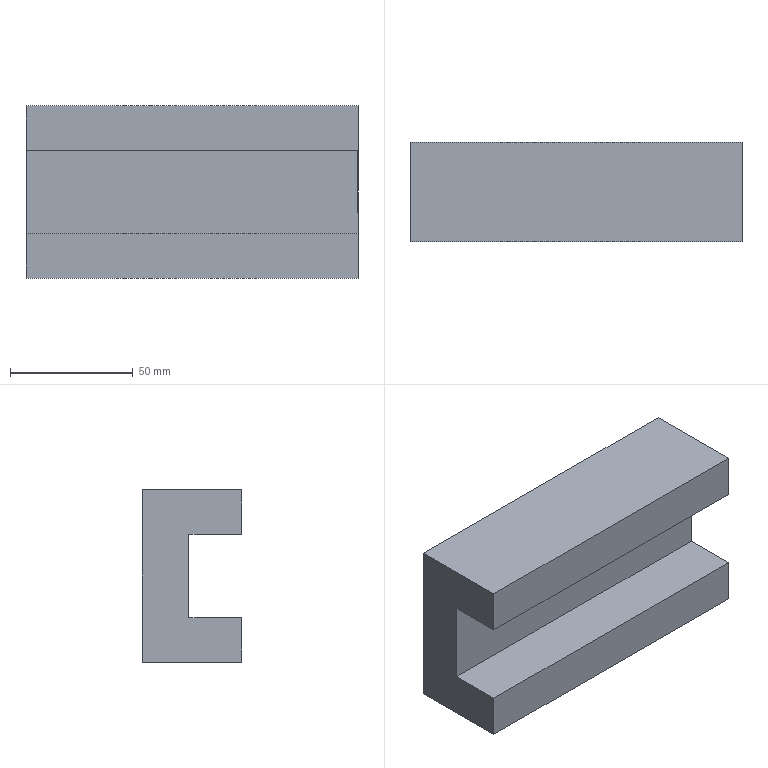Part | SolidWorks | features Cut 2, Extrusion 1 | 1 solid | 22 faces | box 135 x 40.5 x 70 mm | volume 280823 mm3 | plane 14 | cylinder 8 | commonest cylinder face diameters 8 x8
STEP:
#1=CARTESIAN_POINT('',(31.5,24.5,-14.));
#2=VERTEX_POINT('',#1);
#3=CARTESIAN_POINT('',(31.5,24.5,-6.));
#4=VERTEX_POINT('',#3);
#5=CARTESIAN_POINT('',(31.5,24.5,-10.));
#6=DIRECTION('',(0.,1.,0.));
#7=DIRECTION('',(0.,0.,1.));
#8=AXIS2_PLACEMENT_3D('',#5,#6,#7);
#9=CIRCLE('',#8,4.);
#10=EDGE_CURVE('',#2,#4,#9,.T.);
#11=ORIENTED_EDGE('',*,*,#10,.F.);
#12=CARTESIAN_POINT('',(31.5,40.5,-14.));
#13=VERTEX_POINT('',#12);
#14=CARTESIAN_POINT('',(31.5,24.5,-14.));
#15=DIRECTION('',(0.,1.,0.));
#16=VECTOR('',#15,1000.);
#17=LINE('',#14,#16);
#18=EDGE_CURVE('',#2,#13,#17,.T.);
#19=ORIENTED_EDGE('',*,*,#18,.T.);
#20=CARTESIAN_POINT('',(31.5,40.5,-6.));
#21=VERTEX_POINT('',#20);
#22=CARTESIAN_POINT('',(31.5,40.5,-10.));
#23=DIRECTION('',(0.,1.,0.));
#24=DIRECTION('',(0.,0.,1.));
#25=AXIS2_PLACEMENT_3D('',#22,#23,#24);
#26=CIRCLE('',#25,4.);
#27=EDGE_CURVE('',#13,#21,#26,.T.);
#28=ORIENTED_EDGE('',*,*,#27,.T.);
#29=CARTESIAN_POINT('',(31.5,24.5,-6.));
#30=DIRECTION('',(0.,1.,0.));
#31=VECTOR('',#30,1000.);
#32=LINE('',#29,#31);
#33=EDGE_CURVE('',#4,#21,#32,.T.);
#34=ORIENTED_EDGE('',*,*,#33,.F.);
#35=EDGE_LOOP('',(#11,#19,#28,#34));
#36=FACE_OUTER_BOUND('',#35,.T.);
#37=CARTESIAN_POINT('',(31.5,24.5,-10.));
#38=DIRECTION('',(0.,1.,0.));
#39=DIRECTION('',(0.,0.,1.));
#40=AXIS2_PLACEMENT_3D('',#37,#38,#39);
#41=CYLINDRICAL_SURFACE('',#40,4.);
#42=ADVANCED_FACE('',(#36),#41,.F.);
#43=CARTESIAN_POINT('',(31.5,24.5,-64.));
#44=VERTEX_POINT('',#43);
#45=CARTESIAN_POINT('',(31.5,24.5,-56.));
#46=VERTEX_POINT('',#45);
#47=CARTESIAN_POINT('',(31.5,24.5,-60.));
#48=DIRECTION('',(0.,1.,0.));
#49=DIRECTION('',(0.,0.,1.));
#50=AXIS2_PLACEMENT_3D('',#47,#48,#49);
#51=CIRCLE('',#50,4.);
#52=EDGE_CURVE('',#44,#46,#51,.T.);
#53=ORIENTED_EDGE('',*,*,#52,.F.);
#54=CARTESIAN_POINT('',(31.5,40.5,-64.));
#55=VERTEX_POINT('',#54);
#56=CARTESIAN_POINT('',(31.5,24.5,-64.));
#57=DIRECTION('',(0.,1.,0.));
#58=VECTOR('',#57,1000.);
#59=LINE('',#56,#58);
#60=EDGE_CURVE('',#44,#55,#59,.T.);
#61=ORIENTED_EDGE('',*,*,#60,.T.);
#62=CARTESIAN_POINT('',(31.5,40.5,-56.));
#63=VERTEX_POINT('',#62);
#64=CARTESIAN_POINT('',(31.5,40.5,-60.));
#65=DIRECTION('',(0.,1.,0.));
#66=DIRECTION('',(0.,0.,1.));
#67=AXIS2_PLACEMENT_3D('',#64,#65,#66);
#68=CIRCLE('',#67,4.);
#69=EDGE_CURVE('',#55,#63,#68,.T.);
#70=ORIENTED_EDGE('',*,*,#69,.T.);
#71=CARTESIAN_POINT('',(31.5,24.5,-56.));
#72=DIRECTION('',(0.,1.,0.));
#73=VECTOR('',#72,1000.);
#74=LINE('',#71,#73);
#75=EDGE_CURVE('',#46,#63,#74,.T.);
#76=ORIENTED_EDGE('',*,*,#75,.F.);
#77=EDGE_LOOP('',(#53,#61,#70,#76));
#78=FACE_OUTER_BOUND('',#77,.T.);
#79=CARTESIAN_POINT('',(31.5,24.5,-60.));
#80=DIRECTION('',(0.,1.,0.));
#81=DIRECTION('',(0.,0.,1.));
#82=AXIS2_PLACEMENT_3D('',#79,#80,#81);
#83=CYLINDRICAL_SURFACE('',#82,4.);
#84=ADVANCED_FACE('',(#78),#83,.F.);
#85=CARTESIAN_POINT('',(103.5,24.5,-14.));
#86=VERTEX_POINT('',#85);
#87=CARTESIAN_POINT('',(103.5,24.5,-6.));
#88=VERTEX_POINT('',#87);
#89=CARTESIAN_POINT('',(103.5,24.5,-10.));
#90=DIRECTION('',(0.,1.,0.));
#91=DIRECTION('',(0.,0.,1.));
#92=AXIS2_PLACEMENT_3D('',#89,#90,#91);
#93=CIRCLE('',#92,4.);
#94=EDGE_CURVE('',#86,#88,#93,.T.);
#95=ORIENTED_EDGE('',*,*,#94,.F.);
#96=CARTESIAN_POINT('',(103.5,40.5,-14.));
#97=VERTEX_POINT('',#96);
#98=CARTESIAN_POINT('',(103.5,24.5,-14.));
#99=DIRECTION('',(0.,1.,0.));
#100=VECTOR('',#99,1000.);
#101=LINE('',#98,#100);
#102=EDGE_CURVE('',#86,#97,#101,.T.);
#103=ORIENTED_EDGE('',*,*,#102,.T.);
#104=CARTESIAN_POINT('',(103.5,40.5,-6.));
#105=VERTEX_POINT('',#104);
#106=CARTESIAN_POINT('',(103.5,40.5,-10.));
#107=DIRECTION('',(0.,1.,0.));
#108=DIRECTION('',(0.,0.,1.));
#109=AXIS2_PLACEMENT_3D('',#106,#107,#108);
#110=CIRCLE('',#109,4.);
#111=EDGE_CURVE('',#97,#105,#110,.T.);
#112=ORIENTED_EDGE('',*,*,#111,.T.);
#113=CARTESIAN_POINT('',(103.5,24.5,-6.));
#114=DIRECTION('',(0.,1.,0.));
#115=VECTOR('',#114,1000.);
#116=LINE('',#113,#115);
#117=EDGE_CURVE('',#88,#105,#116,.T.);
#118=ORIENTED_EDGE('',*,*,#117,.F.);
#119=EDGE_LOOP('',(#95,#103,#112,#118));
#120=FACE_OUTER_BOUND('',#119,.T.);
#121=CARTESIAN_POINT('',(103.5,24.5,-10.));
#122=DIRECTION('',(0.,1.,0.));
#123=DIRECTION('',(0.,0.,1.));
#124=AXIS2_PLACEMENT_3D('',#121,#122,#123);
#125=CYLINDRICAL_SURFACE('',#124,4.);
#126=ADVANCED_FACE('',(#120),#125,.F.);
#127=CARTESIAN_POINT('',(103.5,24.5,-64.));
#128=VERTEX_POINT('',#127);
#129=CARTESIAN_POINT('',(103.5,24.5,-56.));
#130=VERTEX_POINT('',#129);
#131=CARTESIAN_POINT('',(103.5,24.5,-60.));
#132=DIRECTION('',(0.,1.,0.));
#133=DIRECTION('',(0.,0.,1.));
#134=AXIS2_PLACEMENT_3D('',#131,#132,#133);
#135=CIRCLE('',#134,4.);
#136=EDGE_CURVE('',#128,#130,#135,.T.);
#137=ORIENTED_EDGE('',*,*,#136,.F.);
#138=CARTESIAN_POINT('',(103.5,40.5,-64.));
#139=VERTEX_POINT('',#138);
#140=CARTESIAN_POINT('',(103.5,24.5,-64.));
#141=DIRECTION('',(0.,1.,0.));
#142=VECTOR('',#141,1000.);
#143=LINE('',#140,#142);
#144=EDGE_CURVE('',#128,#139,#143,.T.);
#145=ORIENTED_EDGE('',*,*,#144,.T.);
#146=CARTESIAN_POINT('',(103.5,40.5,-56.));
#147=VERTEX_POINT('',#146);
#148=CARTESIAN_POINT('',(103.5,40.5,-60.));
#149=DIRECTION('',(0.,1.,0.));
#150=DIRECTION('',(0.,0.,1.));
#151=AXIS2_PLACEMENT_3D('',#148,#149,#150);
#152=CIRCLE('',#151,4.);
#153=EDGE_CURVE('',#139,#147,#152,.T.);
#154=ORIENTED_EDGE('',*,*,#153,.T.);
#155=CARTESIAN_POINT('',(103.5,24.5,-56.));
#156=DIRECTION('',(0.,1.,0.));
#157=VECTOR('',#156,1000.);
#158=LINE('',#155,#157);
#159=EDGE_CURVE('',#130,#147,#158,.T.);
#160=ORIENTED_EDGE('',*,*,#159,.F.);
#161=EDGE_LOOP('',(#137,#145,#154,#160));
#162=FACE_OUTER_BOUND('',#161,.T.);
#163=CARTESIAN_POINT('',(103.5,24.5,-60.));
#164=DIRECTION('',(0.,1.,0.));
#165=DIRECTION('',(0.,0.,1.));
#166=AXIS2_PLACEMENT_3D('',#163,#164,#165);
#167=CYLINDRICAL_SURFACE('',#166,4.);
#168=ADVANCED_FACE('',(#162),#167,.F.);
#169=CARTESIAN_POINT('',(0.,0.,-52.));
#170=VERTEX_POINT('',#169);
#171=CARTESIAN_POINT('',(135.,0.,-52.));
#172=VERTEX_POINT('',#171);
#173=CARTESIAN_POINT('',(135.,0.,-52.));
#174=DIRECTION('',(1.,0.,0.));
#175=VECTOR('',#174,1000.);
#176=LINE('',#173,#175);
#177=EDGE_CURVE('',#170,#172,#176,.T.);
#178=ORIENTED_EDGE('',*,*,#177,.F.);
#179=CARTESIAN_POINT('',(0.,0.,-70.));
#180=VERTEX_POINT('',#179);
#181=CARTESIAN_POINT('',(0.,0.,0.));
#182=DIRECTION('',(0.,0.,1.));
#183=VECTOR('',#182,1000.);
#184=LINE('',#181,#183);
#185=EDGE_CURVE('',#180,#170,#184,.T.);
#186=ORIENTED_EDGE('',*,*,#185,.F.);
#187=CARTESIAN_POINT('',(135.,0.,-70.));
#188=VERTEX_POINT('',#187);
#189=CARTESIAN_POINT('',(0.,0.,-70.));
#190=DIRECTION('',(-1.,0.,0.));
#191=VECTOR('',#190,1000.);
#192=LINE('',#189,#191);
#193=EDGE_CURVE('',#188,#180,#192,.T.);
#194=ORIENTED_EDGE('',*,*,#193,.F.);
#195=CARTESIAN_POINT('',(135.,0.,0.));
#196=DIRECTION('',(0.,0.,-1.));
#197=VECTOR('',#196,1000.);
#198=LINE('',#195,#197);
#199=EDGE_CURVE('',#172,#188,#198,.T.);
#200=ORIENTED_EDGE('',*,*,#199,.F.);
#201=EDGE_LOOP('',(#178,#186,#194,#200));
#202=FACE_OUTER_BOUND('',#201,.T.);
#203=CARTESIAN_POINT('',(0.,0.,-70.));
#204=DIRECTION('',(0.,-1.,0.));
#205=DIRECTION('',(0.,0.,-1.));
#206=AXIS2_PLACEMENT_3D('',#203,#204,#205);
#207=PLANE('',#206);
#208=ADVANCED_FACE('',(#202),#207,.T.);
#209=ORIENTED_EDGE('',*,*,#185,.T.);
#210=CARTESIAN_POINT('',(0.,21.5,-52.));
#211=VERTEX_POINT('',#210);
#212=CARTESIAN_POINT('',(0.,21.5,-52.));
#213=DIRECTION('',(0.,-1.,0.));
#214=VECTOR('',#213,1000.);
#215=LINE('',#212,#214);
#216=EDGE_CURVE('',#211,#170,#215,.T.);
#217=ORIENTED_EDGE('',*,*,#216,.F.);
#218=CARTESIAN_POINT('',(0.,21.5,-18.));
#219=VERTEX_POINT('',#218);
#220=CARTESIAN_POINT('',(0.,21.5,-18.));
#221=DIRECTION('',(0.,0.,-1.));
#222=VECTOR('',#221,1000.);
#223=LINE('',#220,#222);
#224=EDGE_CURVE('',#219,#211,#223,.T.);
#225=ORIENTED_EDGE('',*,*,#224,.F.);
#226=CARTESIAN_POINT('',(0.,0.,-18.));
#227=VERTEX_POINT('',#226);
#228=CARTESIAN_POINT('',(0.,21.5,-18.));
#229=DIRECTION('',(0.,-1.,0.));
#230=VECTOR('',#229,1000.);
#231=LINE('',#228,#230);
#232=EDGE_CURVE('',#219,#227,#231,.T.);
#233=ORIENTED_EDGE('',*,*,#232,.T.);
#234=CARTESIAN_POINT('',(0.,0.,0.));
#235=VERTEX_POINT('',#234);
#236=CARTESIAN_POINT('',(0.,0.,0.));
#237=DIRECTION('',(0.,0.,1.));
#238=VECTOR('',#237,1000.);
#239=LINE('',#236,#238);
#240=EDGE_CURVE('',#227,#235,#239,.T.);
#241=ORIENTED_EDGE('',*,*,#240,.T.);
#242=CARTESIAN_POINT('',(0.,40.5,0.));
#243=VERTEX_POINT('',#242);
#244=CARTESIAN_POINT('',(0.,40.5,0.));
#245=DIRECTION('',(0.,-1.,0.));
#246=VECTOR('',#245,1000.);
#247=LINE('',#244,#246);
#248=EDGE_CURVE('',#243,#235,#247,.T.);
#249=ORIENTED_EDGE('',*,*,#248,.F.);
#250=CARTESIAN_POINT('',(0.,40.5,-70.));
#251=VERTEX_POINT('',#250);
#252=CARTESIAN_POINT('',(0.,40.5,0.));
#253=DIRECTION('',(0.,0.,1.));
#254=VECTOR('',#253,1000.);
#255=LINE('',#252,#254);
#256=EDGE_CURVE('',#251,#243,#255,.T.);
#257=ORIENTED_EDGE('',*,*,#256,.F.);
#258=CARTESIAN_POINT('',(0.,40.5,-70.));
#259=DIRECTION('',(0.,-1.,0.));
#260=VECTOR('',#259,1000.);
#261=LINE('',#258,#260);
#262=EDGE_CURVE('',#251,#180,#261,.T.);
#263=ORIENTED_EDGE('',*,*,#262,.T.);
#264=EDGE_LOOP('',(#209,#217,#225,#233,#241,#249,#257,#263));
#265=FACE_OUTER_BOUND('',#264,.T.);
#266=CARTESIAN_POINT('',(0.,40.5,0.));
#267=DIRECTION('',(1.,0.,0.));
#268=DIRECTION('',(0.,0.,-1.));
#269=AXIS2_PLACEMENT_3D('',#266,#267,#268);
#270=PLANE('',#269);
#271=ADVANCED_FACE('',(#265),#270,.F.);
#272=CARTESIAN_POINT('',(135.,0.,0.));
#273=VERTEX_POINT('',#272);
#274=CARTESIAN_POINT('',(0.,0.,0.));
#275=DIRECTION('',(1.,0.,0.));
#276=VECTOR('',#275,1000.);
#277=LINE('',#274,#276);
#278=EDGE_CURVE('',#235,#273,#277,.T.);
#279=ORIENTED_EDGE('',*,*,#278,.T.);
#280=CARTESIAN_POINT('',(135.,40.5,0.));
#281=VERTEX_POINT('',#280);
#282=CARTESIAN_POINT('',(135.,40.5,0.));
#283=DIRECTION('',(0.,-1.,0.));
#284=VECTOR('',#283,1000.);
#285=LINE('',#282,#284);
#286=EDGE_CURVE('',#281,#273,#285,.T.);
#287=ORIENTED_EDGE('',*,*,#286,.F.);
#288=CARTESIAN_POINT('',(0.,40.5,0.));
#289=DIRECTION('',(1.,0.,0.));
#290=VECTOR('',#289,1000.);
#291=LINE('',#288,#290);
#292=EDGE_CURVE('',#243,#281,#291,.T.);
#293=ORIENTED_EDGE('',*,*,#292,.F.);
#294=ORIENTED_EDGE('',*,*,#248,.T.);
#295=EDGE_LOOP('',(#279,#287,#293,#294));
#296=FACE_OUTER_BOUND('',#295,.T.);
#297=CARTESIAN_POINT('',(0.,40.5,0.));
#298=DIRECTION('',(0.,0.,-1.));
#299=DIRECTION('',(-1.,0.,0.));
#300=AXIS2_PLACEMENT_3D('',#297,#298,#299);
#301=PLANE('',#300);
#302=ADVANCED_FACE('',(#296),#301,.F.);
#303=CARTESIAN_POINT('',(135.,21.5,-52.));
#304=VERTEX_POINT('',#303);
#305=CARTESIAN_POINT('',(135.,21.5,-18.));
#306=VERTEX_POINT('',#305);
#307=CARTESIAN_POINT('',(135.,21.5,-18.));
#308=DIRECTION('',(0.,0.,1.));
#309=VECTOR('',#308,1000.);
#310=LINE('',#307,#309);
#311=EDGE_CURVE('',#304,#306,#310,.T.);
#312=ORIENTED_EDGE('',*,*,#311,.F.);
#313=CARTESIAN_POINT('',(135.,21.5,-52.));
#314=DIRECTION('',(0.,-1.,0.));
#315=VECTOR('',#314,1000.);
#316=LINE('',#313,#315);
#317=EDGE_CURVE('',#304,#172,#316,.T.);
#318=ORIENTED_EDGE('',*,*,#317,.T.);
#319=ORIENTED_EDGE('',*,*,#199,.T.);
#320=CARTESIAN_POINT('',(135.,40.5,-70.));
#321=VERTEX_POINT('',#320);
#322=CARTESIAN_POINT('',(135.,40.5,-70.));
#323=DIRECTION('',(0.,-1.,0.));
#324=VECTOR('',#323,1000.);
#325=LINE('',#322,#324);
#326=EDGE_CURVE('',#321,#188,#325,.T.);
#327=ORIENTED_EDGE('',*,*,#326,.F.);
#328=CARTESIAN_POINT('',(135.,40.5,0.));
#329=DIRECTION('',(0.,0.,-1.));
#330=VECTOR('',#329,1000.);
#331=LINE('',#328,#330);
#332=EDGE_CURVE('',#281,#321,#331,.T.);
#333=ORIENTED_EDGE('',*,*,#332,.F.);
#334=ORIENTED_EDGE('',*,*,#286,.T.);
#335=CARTESIAN_POINT('',(135.,0.,-18.));
#336=VERTEX_POINT('',#335);
#337=CARTESIAN_POINT('',(135.,0.,0.));
#338=DIRECTION('',(0.,0.,-1.));
#339=VECTOR('',#338,1000.);
#340=LINE('',#337,#339);
#341=EDGE_CURVE('',#273,#336,#340,.T.);
#342=ORIENTED_EDGE('',*,*,#341,.T.);
#343=CARTESIAN_POINT('',(135.,21.5,-18.));
#344=DIRECTION('',(0.,-1.,0.));
#345=VECTOR('',#344,1000.);
#346=LINE('',#343,#345);
#347=EDGE_CURVE('',#306,#336,#346,.T.);
#348=ORIENTED_EDGE('',*,*,#347,.F.);
#349=EDGE_LOOP('',(#312,#318,#319,#327,#333,#334,#342,#348));
#350=FACE_OUTER_BOUND('',#349,.T.);
#351=CARTESIAN_POINT('',(135.,40.5,0.));
#352=DIRECTION('',(-1.,0.,0.));
#353=DIRECTION('',(0.,0.,1.));
#354=AXIS2_PLACEMENT_3D('',#351,#352,#353);
#355=PLANE('',#354);
#356=ADVANCED_FACE('',(#350),#355,.F.);
#357=ORIENTED_EDGE('',*,*,#193,.T.);
#358=ORIENTED_EDGE('',*,*,#262,.F.);
#359=CARTESIAN_POINT('',(0.,40.5,-70.));
#360=DIRECTION('',(-1.,0.,0.));
#361=VECTOR('',#360,1000.);
#362=LINE('',#359,#361);
#363=EDGE_CURVE('',#321,#251,#362,.T.);
#364=ORIENTED_EDGE('',*,*,#363,.F.);
#365=ORIENTED_EDGE('',*,*,#326,.T.);
#366=EDGE_LOOP('',(#357,#358,#364,#365));
#367=FACE_OUTER_BOUND('',#366,.T.);
#368=CARTESIAN_POINT('',(0.,40.5,-70.));
#369=DIRECTION('',(0.,0.,1.));
#370=DIRECTION('',(1.,0.,0.));
#371=AXIS2_PLACEMENT_3D('',#368,#369,#370);
#372=PLANE('',#371);
#373=ADVANCED_FACE('',(#367),#372,.F.);
#374=CARTESIAN_POINT('',(31.5,40.5,-10.));
#375=DIRECTION('',(0.,1.,0.));
#376=DIRECTION('',(0.,0.,1.));
#377=AXIS2_PLACEMENT_3D('',#374,#375,#376);
#378=CIRCLE('',#377,4.);
#379=EDGE_CURVE('',#21,#13,#378,.T.);
#380=ORIENTED_EDGE('',*,*,#379,.F.);
#381=ORIENTED_EDGE('',*,*,#27,.F.);
#382=EDGE_LOOP('',(#380,#381));
#383=FACE_BOUND('',#382,.T.);
#384=CARTESIAN_POINT('',(31.5,40.5,-60.));
#385=DIRECTION('',(0.,1.,0.));
#386=DIRECTION('',(0.,0.,1.));
#387=AXIS2_PLACEMENT_3D('',#384,#385,#386);
#388=CIRCLE('',#387,4.);
#389=EDGE_CURVE('',#63,#55,#388,.T.);
#390=ORIENTED_EDGE('',*,*,#389,.F.);
#391=ORIENTED_EDGE('',*,*,#69,.F.);
#392=EDGE_LOOP('',(#390,#391));
#393=FACE_BOUND('',#392,.T.);
#394=CARTESIAN_POINT('',(103.5,40.5,-10.));
#395=DIRECTION('',(0.,1.,0.));
#396=DIRECTION('',(0.,0.,1.));
#397=AXIS2_PLACEMENT_3D('',#394,#395,#396);
#398=CIRCLE('',#397,4.);
#399=EDGE_CURVE('',#105,#97,#398,.T.);
#400=ORIENTED_EDGE('',*,*,#399,.F.);
#401=ORIENTED_EDGE('',*,*,#111,.F.);
#402=EDGE_LOOP('',(#400,#401));
#403=FACE_BOUND('',#402,.T.);
#404=CARTESIAN_POINT('',(103.5,40.5,-60.));
#405=DIRECTION('',(0.,1.,0.));
#406=DIRECTION('',(0.,0.,1.));
#407=AXIS2_PLACEMENT_3D('',#404,#405,#406);
#408=CIRCLE('',#407,4.);
#409=EDGE_CURVE('',#147,#139,#408,.T.);
#410=ORIENTED_EDGE('',*,*,#409,.F.);
#411=ORIENTED_EDGE('',*,*,#153,.F.);
#412=EDGE_LOOP('',(#410,#411));
#413=FACE_BOUND('',#412,.T.);
#414=ORIENTED_EDGE('',*,*,#256,.T.);
#415=ORIENTED_EDGE('',*,*,#292,.T.);
#416=ORIENTED_EDGE('',*,*,#332,.T.);
#417=ORIENTED_EDGE('',*,*,#363,.T.);
#418=EDGE_LOOP('',(#414,#415,#416,#417));
#419=FACE_OUTER_BOUND('',#418,.T.);
#420=CARTESIAN_POINT('',(0.,40.5,-70.));
#421=DIRECTION('',(0.,-1.,0.));
#422=DIRECTION('',(0.,0.,-1.));
#423=AXIS2_PLACEMENT_3D('',#420,#421,#422);
#424=PLANE('',#423);
#425=ADVANCED_FACE('',(#383,#393,#403,#413,#419),#424,.F.);
#426=CARTESIAN_POINT('',(135.,0.,-18.));
#427=DIRECTION('',(-1.,0.,0.));
#428=VECTOR('',#427,1000.);
#429=LINE('',#426,#428);
#430=EDGE_CURVE('',#336,#227,#429,.T.);
#431=ORIENTED_EDGE('',*,*,#430,.F.);
#432=ORIENTED_EDGE('',*,*,#341,.F.);
#433=ORIENTED_EDGE('',*,*,#278,.F.);
#434=ORIENTED_EDGE('',*,*,#240,.F.);
#435=EDGE_LOOP('',(#431,#432,#433,#434));
#436=FACE_OUTER_BOUND('',#435,.T.);
#437=CARTESIAN_POINT('',(0.,0.,-70.));
#438=DIRECTION('',(0.,-1.,0.));
#439=DIRECTION('',(0.,0.,-1.));
#440=AXIS2_PLACEMENT_3D('',#437,#438,#439);
#441=PLANE('',#440);
#442=ADVANCED_FACE('',(#436),#441,.T.);
#443=ORIENTED_EDGE('',*,*,#177,.T.);
#444=ORIENTED_EDGE('',*,*,#317,.F.);
#445=CARTESIAN_POINT('',(135.,21.5,-52.));
#446=DIRECTION('',(1.,0.,0.));
#447=VECTOR('',#446,1000.);
#448=LINE('',#445,#447);
#449=EDGE_CURVE('',#211,#304,#448,.T.);
#450=ORIENTED_EDGE('',*,*,#449,.F.);
#451=ORIENTED_EDGE('',*,*,#216,.T.);
#452=EDGE_LOOP('',(#443,#444,#450,#451));
#453=FACE_OUTER_BOUND('',#452,.T.);
#454=CARTESIAN_POINT('',(135.,21.5,-52.));
#455=DIRECTION('',(0.,0.,-1.));
#456=DIRECTION('',(-1.,0.,0.));
#457=AXIS2_PLACEMENT_3D('',#454,#455,#456);
#458=PLANE('',#457);
#459=ADVANCED_FACE('',(#453),#458,.F.);
#460=ORIENTED_EDGE('',*,*,#430,.T.);
#461=ORIENTED_EDGE('',*,*,#232,.F.);
#462=CARTESIAN_POINT('',(135.,21.5,-18.));
#463=DIRECTION('',(-1.,0.,0.));
#464=VECTOR('',#463,1000.);
#465=LINE('',#462,#464);
#466=EDGE_CURVE('',#306,#219,#465,.T.);
#467=ORIENTED_EDGE('',*,*,#466,.F.);
#468=ORIENTED_EDGE('',*,*,#347,.T.);
#469=EDGE_LOOP('',(#460,#461,#467,#468));
#470=FACE_OUTER_BOUND('',#469,.T.);
#471=CARTESIAN_POINT('',(135.,21.5,-18.));
#472=DIRECTION('',(0.,0.,1.));
#473=DIRECTION('',(1.,0.,0.));
#474=AXIS2_PLACEMENT_3D('',#471,#472,#473);
#475=PLANE('',#474);
#476=ADVANCED_FACE('',(#470),#475,.F.);
#477=ORIENTED_EDGE('',*,*,#311,.T.);
#478=ORIENTED_EDGE('',*,*,#466,.T.);
#479=ORIENTED_EDGE('',*,*,#224,.T.);
#480=ORIENTED_EDGE('',*,*,#449,.T.);
#481=EDGE_LOOP('',(#477,#478,#479,#480));
#482=FACE_OUTER_BOUND('',#481,.T.);
#483=CARTESIAN_POINT('',(135.,21.5,-18.));
#484=DIRECTION('',(0.,1.,0.));
#485=DIRECTION('',(0.,0.,1.));
#486=AXIS2_PLACEMENT_3D('',#483,#484,#485);
#487=PLANE('',#486);
#488=ADVANCED_FACE('',(#482),#487,.F.);
#489=ORIENTED_EDGE('',*,*,#144,.F.);
#490=CARTESIAN_POINT('',(103.5,24.5,-60.));
#491=DIRECTION('',(0.,1.,0.));
#492=DIRECTION('',(0.,0.,1.));
#493=AXIS2_PLACEMENT_3D('',#490,#491,#492);
#494=CIRCLE('',#493,4.);
#495=EDGE_CURVE('',#130,#128,#494,.T.);
#496=ORIENTED_EDGE('',*,*,#495,.F.);
#497=ORIENTED_EDGE('',*,*,#159,.T.);
#498=ORIENTED_EDGE('',*,*,#409,.T.);
#499=EDGE_LOOP('',(#489,#496,#497,#498));
#500=FACE_OUTER_BOUND('',#499,.T.);
#501=CARTESIAN_POINT('',(103.5,24.5,-60.));
#502=DIRECTION('',(0.,1.,0.));
#503=DIRECTION('',(0.,0.,1.));
#504=AXIS2_PLACEMENT_3D('',#501,#502,#503);
#505=CYLINDRICAL_SURFACE('',#504,4.);
#506=ADVANCED_FACE('',(#500),#505,.F.);
#507=ORIENTED_EDGE('',*,*,#495,.T.);
#508=ORIENTED_EDGE('',*,*,#136,.T.);
#509=EDGE_LOOP('',(#507,#508));
#510=FACE_OUTER_BOUND('',#509,.T.);
#511=CARTESIAN_POINT('',(103.5,24.5,-60.));
#512=DIRECTION('',(0.,1.,0.));
#513=DIRECTION('',(0.,0.,1.));
#514=AXIS2_PLACEMENT_3D('',#511,#512,#513);
#515=PLANE('',#514);
#516=ADVANCED_FACE('',(#510),#515,.T.);
#517=ORIENTED_EDGE('',*,*,#102,.F.);
#518=CARTESIAN_POINT('',(103.5,24.5,-10.));
#519=DIRECTION('',(0.,1.,0.));
#520=DIRECTION('',(0.,0.,1.));
#521=AXIS2_PLACEMENT_3D('',#518,#519,#520);
#522=CIRCLE('',#521,4.);
#523=EDGE_CURVE('',#88,#86,#522,.T.);
#524=ORIENTED_EDGE('',*,*,#523,.F.);
#525=ORIENTED_EDGE('',*,*,#117,.T.);
#526=ORIENTED_EDGE('',*,*,#399,.T.);
#527=EDGE_LOOP('',(#517,#524,#525,#526));
#528=FACE_OUTER_BOUND('',#527,.T.);
#529=CARTESIAN_POINT('',(103.5,24.5,-10.));
#530=DIRECTION('',(0.,1.,0.));
#531=DIRECTION('',(0.,0.,1.));
#532=AXIS2_PLACEMENT_3D('',#529,#530,#531);
#533=CYLINDRICAL_SURFACE('',#532,4.);
#534=ADVANCED_FACE('',(#528),#533,.F.);
#535=ORIENTED_EDGE('',*,*,#523,.T.);
#536=ORIENTED_EDGE('',*,*,#94,.T.);
#537=EDGE_LOOP('',(#535,#536));
#538=FACE_OUTER_BOUND('',#537,.T.);
#539=CARTESIAN_POINT('',(103.5,24.5,-10.));
#540=DIRECTION('',(0.,1.,0.));
#541=DIRECTION('',(0.,0.,1.));
#542=AXIS2_PLACEMENT_3D('',#539,#540,#541);
#543=PLANE('',#542);
#544=ADVANCED_FACE('',(#538),#543,.T.);
#545=ORIENTED_EDGE('',*,*,#60,.F.);
#546=CARTESIAN_POINT('',(31.5,24.5,-60.));
#547=DIRECTION('',(0.,1.,0.));
#548=DIRECTION('',(0.,0.,1.));
#549=AXIS2_PLACEMENT_3D('',#546,#547,#548);
#550=CIRCLE('',#549,4.);
#551=EDGE_CURVE('',#46,#44,#550,.T.);
#552=ORIENTED_EDGE('',*,*,#551,.F.);
#553=ORIENTED_EDGE('',*,*,#75,.T.);
#554=ORIENTED_EDGE('',*,*,#389,.T.);
#555=EDGE_LOOP('',(#545,#552,#553,#554));
#556=FACE_OUTER_BOUND('',#555,.T.);
#557=CARTESIAN_POINT('',(31.5,24.5,-60.));
#558=DIRECTION('',(0.,1.,0.));
#559=DIRECTION('',(0.,0.,1.));
#560=AXIS2_PLACEMENT_3D('',#557,#558,#559);
#561=CYLINDRICAL_SURFACE('',#560,4.);
#562=ADVANCED_FACE('',(#556),#561,.F.);
#563=ORIENTED_EDGE('',*,*,#551,.T.);
#564=ORIENTED_EDGE('',*,*,#52,.T.);
#565=EDGE_LOOP('',(#563,#564));
#566=FACE_OUTER_BOUND('',#565,.T.);
#567=CARTESIAN_POINT('',(31.5,24.5,-60.));
#568=DIRECTION('',(0.,1.,0.));
#569=DIRECTION('',(0.,0.,1.));
#570=AXIS2_PLACEMENT_3D('',#567,#568,#569);
#571=PLANE('',#570);
#572=ADVANCED_FACE('',(#566),#571,.T.);
#573=ORIENTED_EDGE('',*,*,#18,.F.);
#574=CARTESIAN_POINT('',(31.5,24.5,-10.));
#575=DIRECTION('',(0.,1.,0.));
#576=DIRECTION('',(0.,0.,1.));
#577=AXIS2_PLACEMENT_3D('',#574,#575,#576);
#578=CIRCLE('',#577,4.);
#579=EDGE_CURVE('',#4,#2,#578,.T.);
#580=ORIENTED_EDGE('',*,*,#579,.F.);
#581=ORIENTED_EDGE('',*,*,#33,.T.);
#582=ORIENTED_EDGE('',*,*,#379,.T.);
#583=EDGE_LOOP('',(#573,#580,#581,#582));
#584=FACE_OUTER_BOUND('',#583,.T.);
#585=CARTESIAN_POINT('',(31.5,24.5,-10.));
#586=DIRECTION('',(0.,1.,0.));
#587=DIRECTION('',(0.,0.,1.));
#588=AXIS2_PLACEMENT_3D('',#585,#586,#587);
#589=CYLINDRICAL_SURFACE('',#588,4.);
#590=ADVANCED_FACE('',(#584),#589,.F.);
#591=ORIENTED_EDGE('',*,*,#579,.T.);
#592=ORIENTED_EDGE('',*,*,#10,.T.);
#593=EDGE_LOOP('',(#591,#592));
#594=FACE_OUTER_BOUND('',#593,.T.);
#595=CARTESIAN_POINT('',(31.5,24.5,-10.));
#596=DIRECTION('',(0.,1.,0.));
#597=DIRECTION('',(0.,0.,1.));
#598=AXIS2_PLACEMENT_3D('',#595,#596,#597);
#599=PLANE('',#598);
#600=ADVANCED_FACE('',(#594),#599,.T.);
#601=CLOSED_SHELL('',(#42,#84,#126,#168,#208,#271,#302,#356,#373,#425,#442,#459,#476,#488,#506,#516,#534,#544,#562,#572,#590,#600));
#602=MANIFOLD_SOLID_BREP('',#601);
#603=CARTESIAN_POINT('',(0.,0.,0.));
#604=DIRECTION('',(0.,0.,1.));
#605=DIRECTION('',(1.,0.,0.));
#606=AXIS2_PLACEMENT_3D('',#603,#604,#605);
#607=(LENGTH_UNIT()NAMED_UNIT(*)SI_UNIT(.MILLI.,.METRE.));
#608=UNCERTAINTY_MEASURE_WITH_UNIT(LENGTH_MEASURE(0.00001),#607,'','');
#609=(NAMED_UNIT(*)PLANE_ANGLE_UNIT()SI_UNIT($,.RADIAN.));
#610=(NAMED_UNIT(*)SI_UNIT($,.STERADIAN.)SOLID_ANGLE_UNIT());
#611=(GEOMETRIC_REPRESENTATION_CONTEXT(3)GLOBAL_UNCERTAINTY_ASSIGNED_CONTEXT((#608))GLOBAL_UNIT_ASSIGNED_CONTEXT((#607,#609,#610))REPRESENTATION_CONTEXT('',''));
#612=ADVANCED_BREP_SHAPE_REPRESENTATION('',(#602,#606),#611);